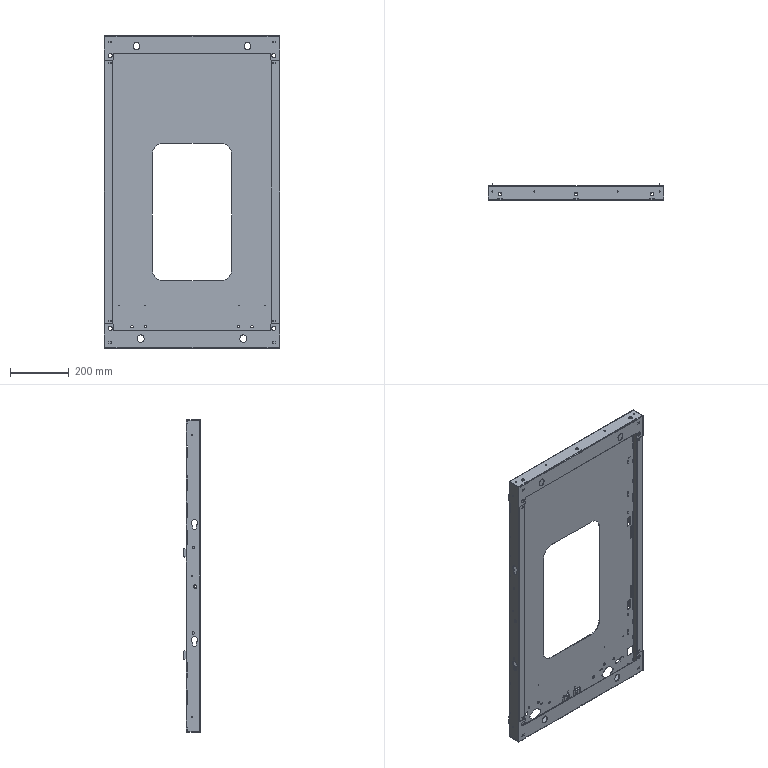Part | NX | features solid 2 | 1 solid | 806 faces | box 600 x 56.705 x 1068 mm | volume 1895264 mm3 | plane 536 | cylinder 212 | torus 24 | cone 20 | spline 14 | commonest cylinder face diameters 5 x40 4 x32 12 x20 0.4 x16 5.4 x16 8.3 x12